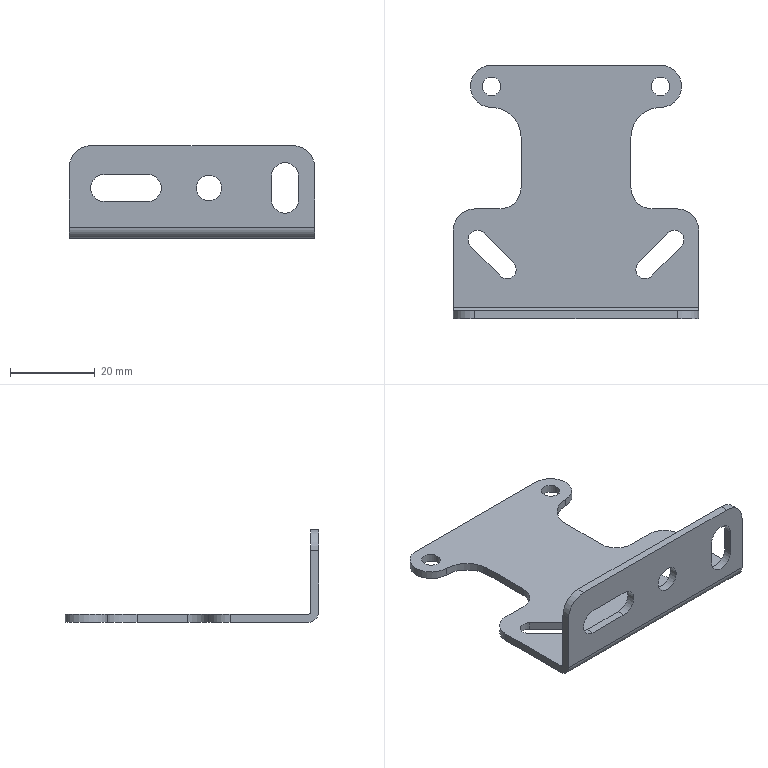Part | STEP file | guangdianzhijia | 1 solid | 43 faces | box 58 x 60 x 21.9 mm | volume 6452 mm3 | cylinder 23 | plane 20 | commonest cylinder face diameters 10 x8 4.4 x6 6.4 x4 14 x2 1.48 x1 5.28 x1